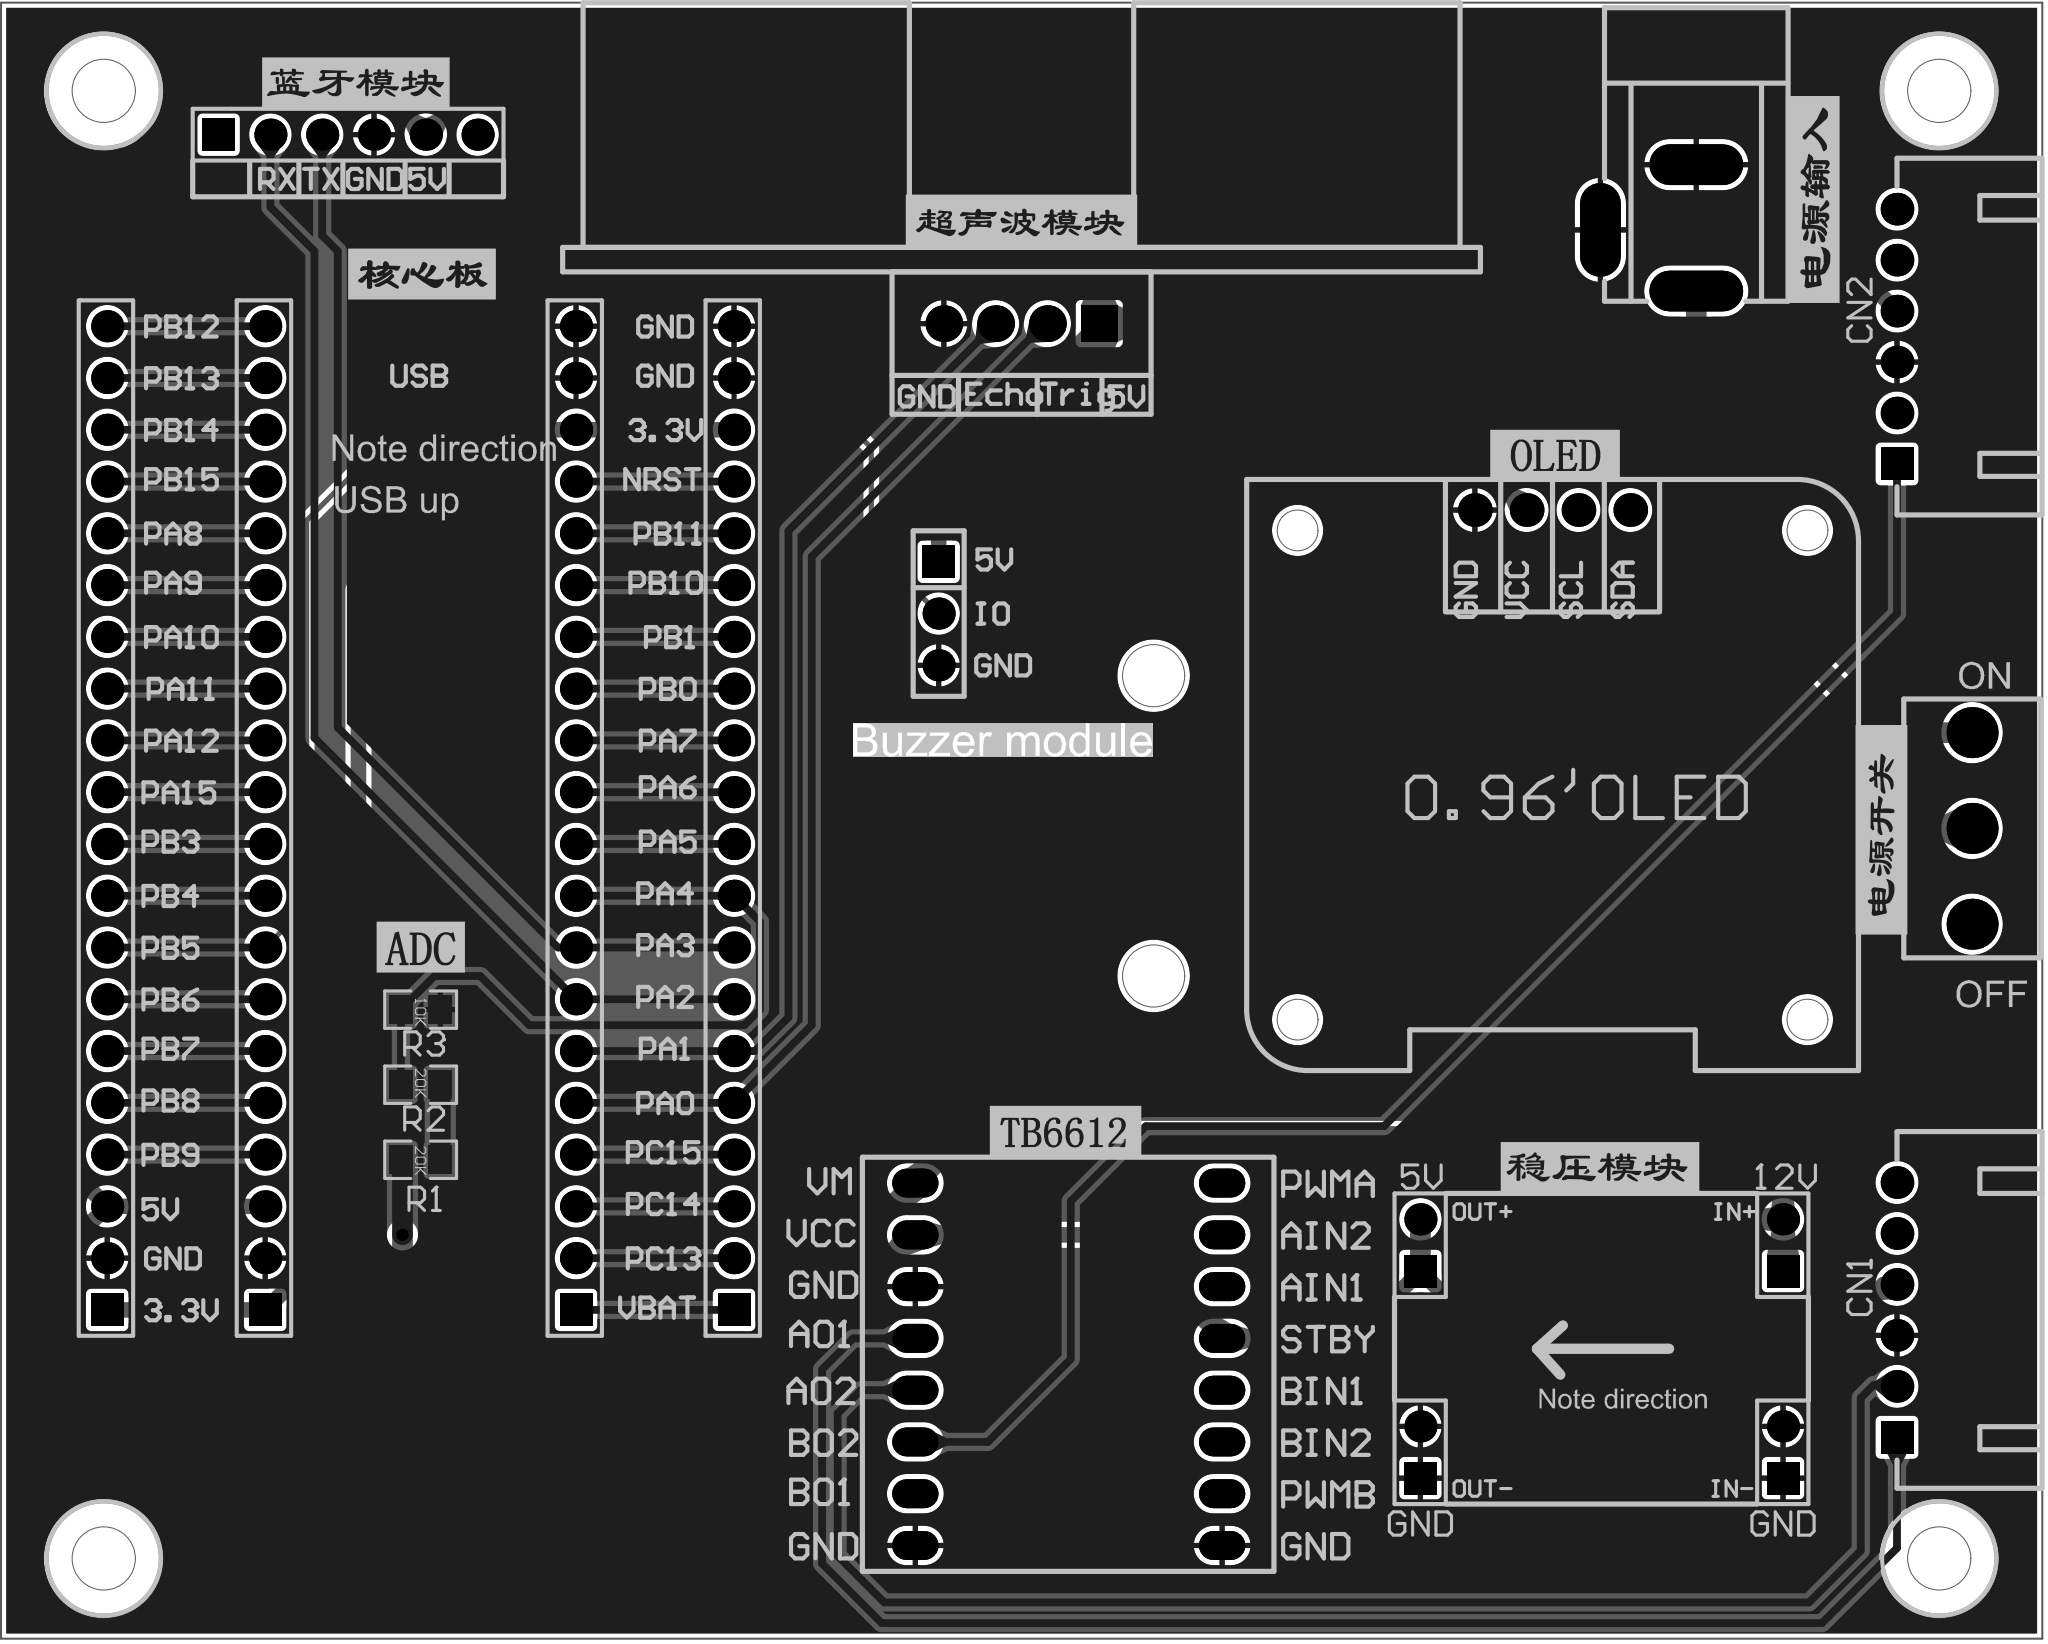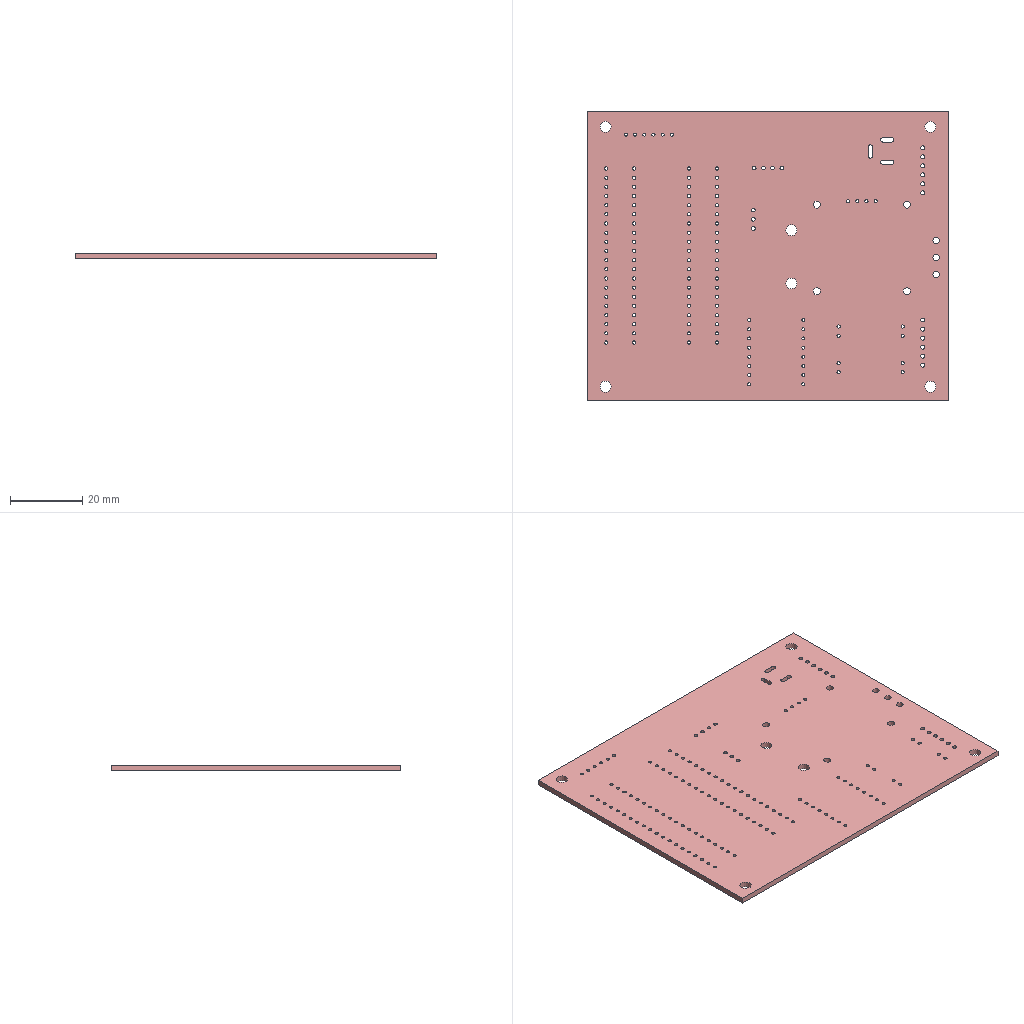Circuit board layout | Altium Designer | box 100.1 x 80.3 x 1.6 mm
Layer stack:
# Altium Designer layer stack of  (unit mm; dielectric type: 0 none, 1 core, 2 prepreg, 3 surface material)
index,name,kind,layer,copper_thickness_mm,dielectric_type,dielectric_thickness_mm,dielectric_material,dielectric_constant
0,Top Paste Mask Layer,other,,,,,,
1,Top Silkscreen Layer,other,,,,,,
2,Top Solder Mask Layer,dielectric,,,3,0.01,,3.3
3,Top Layer,copper,Top Layer,0.035,,,,
4,Dielectric1,dielectric,,,3,0.48,PP,4.5
5,Inner1,copper,Inner1,0.035,,,,
6,Dielectric2,dielectric,,,3,0.48,FR4,4.5
7,Inner2,copper,Inner2,0.035,,,,
8,Dielectric3,dielectric,,,3,0.48,PP,4.5
9,Bottom Layer,copper,Bottom Layer,0.035,,,,
10,Bottom Solder Mask Layer,dielectric,,,3,0.01,,3.3
11,Bottom Silkscreen Layer,other,,,,,,
12,Bottom Paste Mask Layer,other,,,,,,
# drill layer pairs: low layer,high layer
drill_pair,Top Layer,Bottom Layer
Part placement:
Designator,Comment,Layer,Footprint,Center-X(mm),Center-Y(mm),Rotation
CN2,MOTO2,TopLayer,CONN-TH_6P-P2.50_X8821WR-06S-N2SN,175.768,144.399,90
H1,HDR-F-2.54_1x20,TopLayer,HDR-F-2.54_1X20,110.998,120.777,90
H2,HDR-F-2.54_1x20,TopLayer,HDR-F-2.54_1X20,95.758,120.777,90
H4,HDR-F-2.54_1x2,TopLayer,HDR-F-2.54_1X2,170.18,89.662,90
H5,HDR-F-2.54_1x2,TopLayer,HDR-F-2.54_1X2,152.4,99.822,90
H6,HDR-F-2.54_1x2,TopLayer,HDR-F-2.54_1X2,152.4,89.662,90
H9,HDR-F-2.54_1x20,TopLayer,HDR-F-2.54_1X20,118.745,120.777,90
H10,HDR-F-2.54_1x20,TopLayer,HDR-F-2.54_1X20,88.011,120.777,90
H12,,TopLayer,HDR-TH_3P-P2.54-V-F,128.778,130.81,270
R2,20K,TopLayer,R0805,103.378,107.696,0
R3,10K,TopLayer,R0805,103.378,111.379,180
TP2,M3 standoff with silkscreen,TopLayer,M3铜柱,0,0,0
TP3,M3 standoff with silkscreen,TopLayer,M3铜柱,0,0,0
TP4,M3 standoff with silkscreen,TopLayer,M3铜柱,0,0,0
NO,MODULE_HC-SR04,TopLayer,HC-SR04,132.842,145.034,180
DC1,DC005_C431533,TopLayer,DC-IN-TH_DC005,163.576,149.733,270
H3,HDR-F-2.54_1x2,TopLayer,HDR-F-2.54_1X2,170.18,99.822,90
H11,Bluetooth,TopLayer,HDR-F-2.54_1X6,99.822,154.305,0
P1,0.96OLED_4P,TopLayer,0.96OLED_4P,158.88,135.889,0
R1,20K,TopLayer,R0805,103.378,104.013,180
SW3,SS-12D10L5,TopLayer,SW-TH_SS-12D10L5,179.451,120.269,270
TP1,M3 standoff with silkscreen,TopLayer,M3铜柱,0,0,0
U1,TB6612FNG component,TopLayer,TB6612FNG封装,135.156,93.98,0
CN1,MOTO1,TopLayer,CONN-TH_6P-P2.50_X8821WR-06S-N2SN,175.768,96.647,90
Pad and via stacks:
# Altium Designer via and pad stacks of  (unit mm). Each distinct definition once, with the count of objects using it.
# via: kind,start_layer,end_layer,hole_mm,diameter_mm,mode(0 simple;1 top-mid-bottom;2 full stack),diameter_per_layer,count,example_net
# pad: kind,layer,hole_mm,hole_type(0 round;1 square;2 slot),plating,top_size,top_shape(1 round;2 rect;3 octagon;9 rounded rect),mid_size,bottom_size,mode,footprint,size_per_layer,count,example
pad,Multi-Layer,1.1,0,plated,1.6x1.6,1,1.6x1.6,1.6x1.6,0,CONN-TH_6P-P2.50_X8821WR-06S-N2SN,,10,CN2.6
pad,Multi-Layer,1.1,0,plated,1.6x1.6,2,1.6x1.6,1.6x1.6,0,CONN-TH_6P-P2.50_X8821WR-06S-N2SN,,2,CN2.1
pad,Multi-Layer,0.889,0,plated,1.575x1.575,1,1.575x1.575,1.575x1.575,0,HDR-F-2.54_1X20,,76,H1.20
pad,Multi-Layer,0.889,0,plated,1.575x1.575,2,1.575x1.575,1.575x1.575,0,HDR-F-2.54_1X20,,4,H1.1
pad,Multi-Layer,0.889,0,plated,1.575x1.575,2,1.575x1.575,1.575x1.575,0,HDR-F-2.54_1X2,,4,H4.1
pad,Multi-Layer,0.889,0,plated,1.575x1.575,1,1.575x1.575,1.575x1.575,0,HDR-F-2.54_1X2,,4,H4.2
pad,Multi-Layer,1.02,0,plated,1.575x1.575,1,1.575x1.575,1.575x1.575,0,HDR-TH_3P-P2.54-V-F,,2,H12.3
pad,Multi-Layer,1.02,0,plated,1.575x1.575,2,1.575x1.575,1.575x1.575,0,HDR-TH_3P-P2.54-V-F,,1,H12.1
pad,Multi-Layer,1,0,plated,1.8x1.8,1,1.8x1.8,1.8x1.8,0,HC-SR04,,3,NO.4
pad,Multi-Layer,1,0,plated,1.8x1.8,2,1.8x1.8,1.8x1.8,0,HC-SR04,,1,NO.1
pad,Multi-Layer,1.2,2,plated,2x4.6,1,2x4.6,2x4.6,0,DC-IN-TH_DC005,,2,DC1.1
pad,Multi-Layer,1.2,2,plated,4.6x2,1,4.6x2,4.6x2,0,DC-IN-TH_DC005,,1,DC1.3
pad,Multi-Layer,0.889,0,plated,1.575x1.575,1,1.575x1.575,1.575x1.575,0,HDR-F-2.54_1X6,,5,H11.6
pad,Multi-Layer,0.889,0,plated,1.575x1.575,2,1.575x1.575,1.575x1.575,0,HDR-F-2.54_1X6,,1,H11.1
pad,Multi-Layer,0.89,0,plated,1.65x1.65,1,1.65x1.65,1.65x1.65,0,0.96OLED_4P,,4,P1.1
pad,Multi-Layer,1.8,0,plated,2.5x2.5,1,2.5x2.5,2.5x2.5,0,SW-TH_SS-12D10L5,,3,SW3.1
pad,Multi-Layer,0.8499,2,plated,2.276x1.422,1,2.276x1.422,2.276x1.422,0,TB6612FNG\u00B7\u00E2\u00D7\u00B0,,16,U1.1
pad,Top Layer,0,0,plated,1.133x1.377,2,1.133x1.377,1.133x1.377,0,R0805,,6,R2.2
via,Top Layer,Bottom Layer,0.3048,0.6096,0,,1,VBAT_IN
Copper pours:
name,layer,net,type(0 solid;1 hatched;2 none)
Bottom Layer-GND,Bottom Layer,GND,0
Inner1-GND,Inner1,GND,0
Inner2-GND,Inner2,GND,0
Top Layer-GND,Top Layer,GND,0
Design rules, without the lines most boards share:
# Altium Designer design rules of  (exported by Altium Designer, unit mm)
# columns: name | kind | enabled | priority | scope1 | scope2 | descriptor | typed fields (field=value)
Plane_innerPlane | 0 | disabled | 1 | All | All | Clearance Constraint (Gap=6mil) (Disabled)(All),(All) | gap=0.1524
Plane_innerPlane_1 | 63 | disabled | 1 | All | All | Board Clearance Constraint (Gap=0mil) (Disabled)(All) |
Copper_copperRegion | 0 | disabled | 2 | All | All | Clearance Constraint (Gap=6mil) (Disabled)(All),(All) | gap=0.1524
Copper_copperRegion_1 | 63 | disabled | 2 | All | All | Board Clearance Constraint (Gap=0mil) (Disabled)(All) |
Copper_gge61610 | 0 | disabled | 3 | All | All | Clearance Constraint (Gap=6mil) (Disabled)(All),(All) | gap=0.1524
Copper_gge61610_1 | 63 | disabled | 3 | All | All | Board Clearance Constraint (Gap=0mil) (Disabled)(All) |
Copper_gge61631 | 0 | disabled | 4 | All | All | Clearance Constraint (Gap=6mil) (Disabled)(All),(All) | gap=0.1524
Copper_gge61631_1 | 63 | disabled | 4 | All | All | Board Clearance Constraint (Gap=0mil) (Disabled)(All) |
Copper_gge61637 | 0 | disabled | 5 | All | All | Clearance Constraint (Gap=6mil) (Disabled)(All),(All) | gap=0.1524
Copper_gge61637_1 | 63 | disabled | 5 | All | All | Board Clearance Constraint (Gap=0mil) (Disabled)(All) |
Copper_gge61622(1) | 0 | disabled | 6 | All | All | Clearance Constraint (Gap=6mil) (Disabled)(All),(All) | gap=0.1524
Copper_gge61622(1)_1 | 63 | disabled | 6 | All | All | Board Clearance Constraint (Gap=0mil) (Disabled)(All) |
safeClearance | 0 | enabled | 7 | All | All | Clearance Constraint (Gap=6mil) (All),(All) | gap=0.1524
safeClearance_1 | 63 | enabled | 7 | All | All | Board Clearance Constraint (Gap=0mil) (All) |
gge61610 | 52 | disabled | 1 | All | All | Hole To Hole Clearance (Gap=0mil) (Disabled)(All),(All) | gap=0
gge61631 | 52 | disabled | 2 | All | All | Hole To Hole Clearance (Gap=0mil) (Disabled)(All),(All) | gap=0
gge61637 | 52 | disabled | 3 | All | All | Hole To Hole Clearance (Gap=0mil) (Disabled)(All),(All) | gap=0
gge61622 | 52 | disabled | 4 | All | All | Hole To Hole Clearance (Gap=0mil) (Disabled)(All),(All) | gap=0
gge61622(1) | 52 | disabled | 5 | All | All | Hole To Hole Clearance (Gap=0mil) (Disabled)(All),(All) | gap=0
Common | 52 | enabled | 6 | All | All | Hole To Hole Clearance (Gap=11.8mil) (All),(All) | gap=0.2997
trackWidth | 2 | enabled | 1 | All | All | Width Constraint (Min=5mil) (Max=100mil) (Preferred=10mil) (All) |
viaSize | 11 | enabled | 1 | All | All | Routing Via (MinHoleWidth=11.811mil) (MaxHoleWidth=236.22mil) (PreferredHoleWidth=12.008mil) (MinWidth=19.685mil) (MaxWidth=393.701mil) (PreferedWidth=24.016mil) (All) | via_min_hole=0.3 via_max_hole=6 via_preferred_diameter=0.61 via_preferred_hole=0.305
gge61610_1 | 20 | disabled | 1 | All | All | Polygon Connect Rule(Relief Connect )(Conductor Width=10mil) (Relief Angle=90 Angle) (Entries=4) (Air Gap Width=10mil) (Disabled)(All),(All) | connect_style(0=relief,1=direct,2=none)=0 relief_conductor_width=0.254 relief_entries=4
gge61631_1 | 20 | disabled | 2 | All | All | Polygon Connect Rule(Relief Connect )(Conductor Width=10mil) (Relief Angle=90 Angle) (Entries=4) (Air Gap Width=10mil) (Disabled)(All),(All) | connect_style(0=relief,1=direct,2=none)=0 relief_conductor_width=0.254 relief_entries=4
gge61637_1 | 20 | disabled | 3 | All | All | Polygon Connect Rule(Relief Connect )(Conductor Width=10mil) (Relief Angle=90 Angle) (Entries=4) (Air Gap Width=10mil) (Disabled)(All),(All) | connect_style(0=relief,1=direct,2=none)=0 relief_conductor_width=0.254 relief_entries=4
gge61622(1)_1 | 20 | disabled | 4 | All | All | Polygon Connect Rule(Relief Connect )(Conductor Width=10mil) (Relief Angle=90 Angle) (Entries=4) (Air Gap Width=10mil) (Disabled)(All),(All) | connect_style(0=relief,1=direct,2=none)=0 relief_conductor_width=0.254 relief_entries=4
copperRegion | 20 | enabled | 5 | All | All | Polygon Connect Rule(Relief Connect )(Conductor Width=10mil) (Relief Angle=90 Angle) (Entries=4) (Air Gap Width=10mil) (All),(All) | connect_style(0=relief,1=direct,2=none)=0 relief_conductor_width=0.254 relief_entries=4